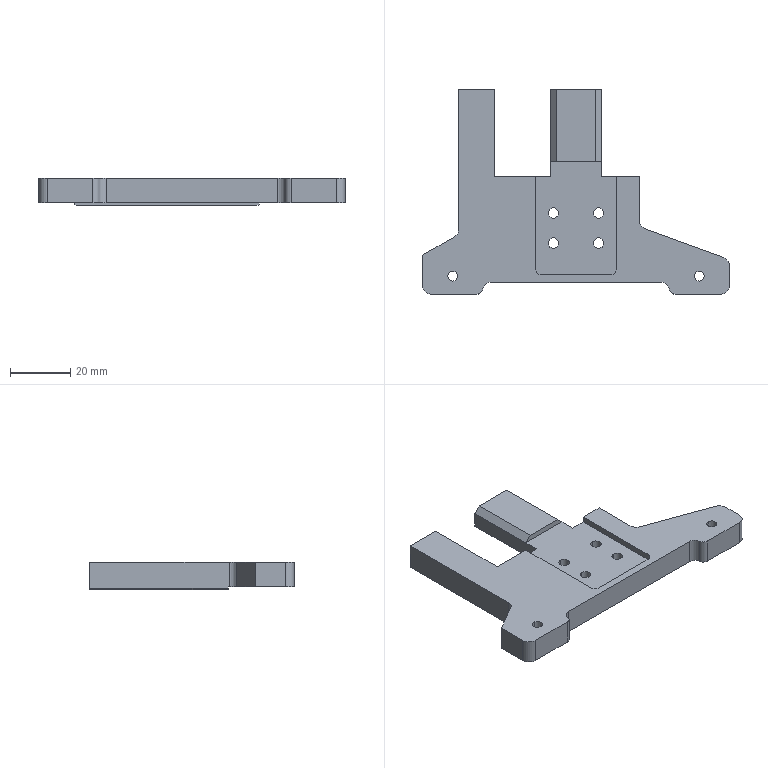NC program | NX | posted with a generic post | part box 102 x 68 x 9.2 mm
Whole program:
N10 G17 G21 G94 G90
(ZLEVEL_PROFILE_COPY_1 , TOOL : D4)
N12 T04 M6
N14 G54
N16 G17 G0 G90 X-43.633 Y-13.513 S7000 M3
N18 G43 Z11. H4
N20 Z-0.5
N22 G94 G1 X-43.033 Y-13.86 F1000.
N24 G3 X-42.633 Y-13.86 R0.4
N26 G1 X-41.5 Y-13.206 F1500.
N28 G3 X-41. Y-12.34 R1.
N30 G1 Y-11.032
N32 G3 X-41.2 Y-10.686 R0.4
N34 G1 X-41.8 Y-10.339
N36 G0 X-43.633 Y-13.513 Z-1.
N38 G1 X-43.033 Y-13.86 F1000.
N40 G3 X-42.633 Y-13.86 R0.4
N42 G1 X-41.5 Y-13.206 F1500.
N44 G3 X-41. Y-12.34 R1.
N46 G1 Y-11.032
N48 G3 X-41.2 Y-10.686 R0.4
N50 G1 X-41.8 Y-10.339
N52 G0 X-43.633 Y-13.513 Z-1.5
N54 G1 X-43.033 Y-13.86 F1000.
N56 G3 X-42.633 Y-13.86 R0.4
N58 G1 X-41.5 Y-13.206 F1500.
N60 G3 X-41. Y-12.34 R1.
N62 G1 Y-11.032
N64 G3 X-41.2 Y-10.686 R0.4
N66 G1 X-41.8 Y-10.339
N68 G0 X-43.633 Y-13.513 Z-2.
N70 G1 X-43.033 Y-13.86 F1000.
N72 G3 X-42.633 Y-13.86 R0.4
N74 G1 X-41.5 Y-13.206 F1500.
N76 G3 X-41. Y-12.34 R1.
N78 G1 Y-11.032
N80 G3 X-41.2 Y-10.686 R0.4
N82 G1 X-41.8 Y-10.339
N84 G0 X-43.633 Y-13.513 Z-2.48
N86 G1 X-43.033 Y-13.86 F1000.
N88 G3 X-42.633 Y-13.86 R0.4
N90 G1 X-41.5 Y-13.206 F1500.
N92 G3 X-41. Y-12.34 R1.
N94 G1 Y-11.032
N96 G3 X-41.2 Y-10.686 R0.4
N98 G1 X-41.8 Y-10.339
N100 G0 X-43.633 Y-13.513 Z-2.96
N102 G1 X-43.033 Y-13.86 F1000.
N104 G3 X-42.633 Y-13.86 R0.4
N106 G1 X-41.5 Y-13.206 F1500.
N108 G3 X-41. Y-12.34 R1.
N110 G1 Y-11.032
N112 G3 X-41.2 Y-10.686 R0.4
N114 G1 X-41.8 Y-10.339
N116 G0 X-43.633 Y-13.513 Z-3.44
N118 G1 X-43.033 Y-13.86 F1000.
N120 G3 X-42.633 Y-13.86 R0.4
N122 G1 X-41.5 Y-13.206 F1500.
N124 G3 X-41. Y-12.34 R1.
N126 G1 Y-11.032
N128 G3 X-41.2 Y-10.686 R0.4
N130 G1 X-41.8 Y-10.339
N132 G0 X-43.633 Y-13.513 Z-3.92
N134 G1 X-43.033 Y-13.86 F1000.
N136 G3 X-42.633 Y-13.86 R0.4
N138 G1 X-41.5 Y-13.206 F1500.
N140 G3 X-41. Y-12.34 R1.
N142 G1 Y-11.032
N144 G3 X-41.2 Y-10.686 R0.4
N146 G1 X-41.8 Y-10.339
N148 G0 X-43.633 Y-13.513 Z-4.4
N150 G1 X-43.033 Y-13.86 F1000.
N152 G3 X-42.633 Y-13.86 R0.4
N154 G1 X-41.5 Y-13.206 F1500.
N156 G3 X-41. Y-12.34 R1.
N158 G1 Y-11.032
N160 G3 X-41.2 Y-10.686 R0.4
N162 G1 X-41.8 Y-10.339
N164 G0 X-43.633 Y-13.513 Z-4.88
N166 G1 X-43.033 Y-13.86 F1000.
N168 G3 X-42.633 Y-13.86 R0.4
N170 G1 X-41.5 Y-13.206 F1500.
N172 G3 X-41. Y-12.34 R1.
N174 G1 Y-11.032
N176 G3 X-41.2 Y-10.686 R0.4
N178 G1 X-41.8 Y-10.339
N180 G0 X-43.633 Y-13.513 Z-5.36
N182 G1 X-43.033 Y-13.86 F1000.
N184 G3 X-42.633 Y-13.86 R0.4
N186 G1 X-41.5 Y-13.206 F1500.
N188 G3 X-41. Y-12.34 R1.
N190 G1 Y-11.032
N192 G3 X-41.2 Y-10.686 R0.4
N194 G1 X-41.8 Y-10.339
N196 G0 X-43.633 Y-13.513 Z-5.84
N198 G1 X-43.033 Y-13.86 F1000.
N200 G3 X-42.633 Y-13.86 R0.4
N202 G1 X-41.5 Y-13.206 F1500.
N204 G3 X-41. Y-12.34 R1.
N206 G1 Y-11.032
N208 G3 X-41.2 Y-10.686 R0.4
N210 G1 X-41.8 Y-10.339
N212 G0 X-43.633 Y-13.513 Z-6.32
N214 G1 X-43.033 Y-13.86 F1000.
N216 G3 X-42.633 Y-13.86 R0.4
N218 G1 X-41.5 Y-13.206 F1500.
N220 G3 X-41. Y-12.34 R1.
N222 G1 Y-11.032
N224 G3 X-41.2 Y-10.686 R0.4
N226 G1 X-41.8 Y-10.339
N228 G0 X-43.633 Y-13.513 Z-6.8
N230 G1 X-43.033 Y-13.86 F1000.
N232 G3 X-42.633 Y-13.86 R0.4
N234 G1 X-41.5 Y-13.206 F1500.
N236 G3 X-41. Y-12.34 R1.
N238 G1 Y-11.032
N240 G3 X-41.2 Y-10.686 R0.4
N242 G1 X-41.8 Y-10.339
N244 G0 X-43.633 Y-13.513 Z-7.28
N246 G1 X-43.033 Y-13.86 F1000.
N248 G3 X-42.633 Y-13.86 R0.4
N250 G1 X-41.5 Y-13.206 F1500.
N252 G3 X-41. Y-12.34 R1.
N254 G1 Y-11.032
N256 G3 X-41.2 Y-10.686 R0.4
N258 G1 X-41.8 Y-10.339
N260 G0 X-43.633 Y-13.513 Z-7.76
N262 G1 X-43.033 Y-13.86 F1000.
N264 G3 X-42.633 Y-13.86 R0.4
N266 G1 X-41.5 Y-13.206 F1500.
N268 G3 X-41. Y-12.34 R1.
N270 G1 Y-11.032
N272 G3 X-41.2 Y-10.686 R0.4
N274 G1 X-41.8 Y-10.339
N276 G0 X-43.633 Y-13.513 Z-8.24
N278 G1 X-43.033 Y-13.86 F1000.
N280 G3 X-42.633 Y-13.86 R0.4
N282 G1 X-41.5 Y-13.206 F1500.
N284 G3 X-41. Y-12.34 R1.
N286 G1 Y-11.032
N288 G3 X-41.2 Y-10.686 R0.4
N290 G1 X-41.8 Y-10.339
N292 G0 X-43.637 Y-13.516 Z-8.72
N294 G1 X-43.037 Y-13.862 F1000.
N296 G3 X-42.637 Y-13.862 R0.4
N298 G1 X-41.5 Y-13.206 F1500.
N300 G3 X-41. Y-12.34 R1.
N302 G1 Y-11.031
N304 G3 X-41.2 Y-10.685 R0.4
N306 G1 X-41.8 Y-10.339
N308 G0 X-43.637 Y-13.516 Z-9.2
N310 G1 X-43.037 Y-13.862 F1000.
N312 G3 X-42.637 Y-13.862 R0.4
N314 G1 X-41.5 Y-13.206 F1500.
N316 G3 X-41. Y-12.34 R1.
N318 G1 Y-11.031
N320 G3 X-41.2 Y-10.685 R0.4
N322 G1 X-41.8 Y-10.339
N324 G0 Z11.
N326 X-24.2 Y10.846
N328 Z-0.5
N330 G1 X-24.8 Y10.499 F1000.
N332 G3 X-25. Y10.153 R0.4
N334 G1 Y7. F1500.
N336 X-21.847
N338 G3 X-21.501 Y7.2 R0.4
N340 G1 X-21.154 Y7.8
N342 G0 X-24.2 Y10.846 Z-1.
N344 G1 X-24.8 Y10.499 F1000.
N346 G3 X-25. Y10.153 R0.4
N348 G1 Y7. F1500.
N350 X-21.847
N352 G3 X-21.501 Y7.2 R0.4
N354 G1 X-21.154 Y7.8
N356 G0 X-24.2 Y10.846 Z-1.5
N358 G1 X-24.8 Y10.499 F1000.
N360 G3 X-25. Y10.153 R0.4
N362 G1 Y7. F1500.
N364 X-21.847
N366 G3 X-21.501 Y7.2 R0.4
N368 G1 X-21.154 Y7.8
N370 G0 X-24.2 Y10.846 Z-2.
N372 G1 X-24.8 Y10.499 F1000.
N374 G3 X-25. Y10.153 R0.4
N376 G1 Y7. F1500.
N378 X-21.847
N380 G3 X-21.501 Y7.2 R0.4
N382 G1 X-21.154 Y7.8
N384 G0 X-24.2 Y10.846 Z-2.48
N386 G1 X-24.8 Y10.499 F1000.
N388 G3 X-25. Y10.153 R0.4
N390 G1 Y7. F1500.
N392 X-21.847
N394 G3 X-21.501 Y7.2 R0.4
N396 G1 X-21.154 Y7.8
N398 G0 X-24.2 Y10.846 Z-2.96
N400 G1 X-24.8 Y10.499 F1000.
N402 G3 X-25. Y10.153 R0.4
N404 G1 Y7. F1500.
N406 X-21.847
N408 G3 X-21.501 Y7.2 R0.4
N410 G1 X-21.154 Y7.8
N412 G0 X-24.2 Y10.846 Z-3.44
N414 G1 X-24.8 Y10.499 F1000.
N416 G3 X-25. Y10.153 R0.4
N418 G1 Y7. F1500.
N420 X-21.847
N422 G3 X-21.501 Y7.2 R0.4
N424 G1 X-21.154 Y7.8
N426 G0 X-24.2 Y10.846 Z-3.92
N428 G1 X-24.8 Y10.499 F1000.
N430 G3 X-25. Y10.153 R0.4
N432 G1 Y7. F1500.
N434 X-21.847
N436 G3 X-21.501 Y7.2 R0.4
N438 G1 X-21.154 Y7.8
N440 G0 X-24.2 Y10.846 Z-4.4
N442 G1 X-24.8 Y10.499 F1000.
N444 G3 X-25. Y10.153 R0.4
N446 G1 Y7. F1500.
N448 X-21.847
N450 G3 X-21.501 Y7.2 R0.4
N452 G1 X-21.154 Y7.8
N454 G0 X-24.2 Y10.846 Z-4.88
N456 G1 X-24.8 Y10.499 F1000.
N458 G3 X-25. Y10.153 R0.4
N460 G1 Y7. F1500.
N462 X-21.847
N464 G3 X-21.501 Y7.2 R0.4
N466 G1 X-21.154 Y7.8
N468 G0 X-24.2 Y10.846 Z-5.36
N470 G1 X-24.8 Y10.499 F1000.
N472 G3 X-25. Y10.153 R0.4
N474 G1 Y7. F1500.
N476 X-21.847
N478 G3 X-21.501 Y7.2 R0.4
N480 G1 X-21.154 Y7.8
N482 G0 X-24.2 Y10.846 Z-5.84
N484 G1 X-24.8 Y10.499 F1000.
N486 G3 X-25. Y10.153 R0.4
N488 G1 Y7. F1500.
N490 X-21.847
N492 G3 X-21.501 Y7.2 R0.4
N494 G1 X-21.154 Y7.8
N496 G0 X-24.2 Y10.846 Z-6.32
N498 G1 X-24.8 Y10.499 F1000.
N500 G3 X-25. Y10.153 R0.4
N502 G1 Y7. F1500.
N504 X-21.847
N506 G3 X-21.501 Y7.2 R0.4
N508 G1 X-21.154 Y7.8
N510 G0 X-24.2 Y10.846 Z-6.8
N512 G1 X-24.8 Y10.499 F1000.
N514 G3 X-25. Y10.153 R0.4
N516 G1 Y7. F1500.
N518 X-21.847
N520 G3 X-21.501 Y7.2 R0.4
N522 G1 X-21.154 Y7.8
N524 G0 X-24.2 Y10.846 Z-7.28
N526 G1 X-24.8 Y10.499 F1000.
N528 G3 X-25. Y10.153 R0.4
N530 G1 Y7. F1500.
N532 X-21.847
N534 G3 X-21.501 Y7.2 R0.4
N536 G1 X-21.154 Y7.8
N538 G0 X-24.2 Y10.846 Z-7.76
N540 G1 X-24.8 Y10.499 F1000.
N542 G3 X-25. Y10.153 R0.4
N544 G1 Y7. F1500.
N546 X-21.847
N548 G3 X-21.501 Y7.2 R0.4
N550 G1 X-21.154 Y7.8
N552 G0 X-24.2 Y10.846 Z-8.24
N554 G1 X-24.8 Y10.499 F1000.
N556 G3 X-25. Y10.153 R0.4
N558 G1 Y7. F1500.
N560 X-21.847
N562 G3 X-21.501 Y7.2 R0.4
N564 G1 X-21.154 Y7.8
N566 G0 X-24.2 Y10.846 Z-8.72
N568 G1 X-24.8 Y10.499 F1000.
N570 G3 X-25. Y10.153 R0.4
N572 G1 Y7. F1500.
N574 X-21.847
N576 G3 X-21.501 Y7.2 R0.4
N578 G1 X-21.154 Y7.8
N580 G0 X-24.2 Y10.846 Z-9.2
N582 G1 X-24.8 Y10.499 F1000.
N584 G3 X-25. Y10.153 R0.4
N586 G1 Y7. F1500.
N588 X-21.847
N590 G3 X-21.501 Y7.2 R0.4
N592 G1 X-21.154 Y7.8
N594 G0 Z11.
N596 X-10.7 Y-21.654
N598 Z-0.5
N600 G1 X-11.3 Y-22.001 F1000.
N602 G3 X-11.5 Y-22.347 R0.4
N604 G1 Y-25.5 F1500.
N606 X-8.347
N608 G3 X-8.001 Y-25.3 R0.4
N610 G1 X-7.654 Y-24.7
N612 G0 X-10.7 Y-21.654 Z-1.
N614 G1 X-11.3 Y-22.001 F1000.
N616 G3 X-11.5 Y-22.347 R0.4
N618 G1 Y-25.5 F1500.
N620 X-8.347
N622 G3 X-8.001 Y-25.3 R0.4
N624 G1 X-7.654 Y-24.7
N626 G0 X-10.7 Y-21.654 Z-1.5
N628 G1 X-11.3 Y-22.001 F1000.
N630 G3 X-11.5 Y-22.347 R0.4
N632 G1 Y-25.5 F1500.
N634 X-8.347
N636 G3 X-8.001 Y-25.3 R0.4
N638 G1 X-7.654 Y-24.7
N640 G0 X-10.7 Y-21.654 Z-2.
N642 G1 X-11.3 Y-22.001 F1000.
N644 G3 X-11.5 Y-22.347 R0.4
N646 G1 X-11.499 Y-25.5 F1500.
N648 X-8.347
N650 G3 X-8.001 Y-25.3 R0.4
N652 G1 X-7.654 Y-24.7
N654 G0 Z11.
N656 X7.654
N658 Z-0.5
N660 G1 X8. Y-25.3 F1000.
N662 G3 X8.347 Y-25.5 R0.4
N664 G1 X11.5 F1500.
N666 Y-22.347
N668 G3 X11.3 Y-22. R0.4
N670 G1 X10.7 Y-21.654
N672 G0 X7.654 Y-24.7 Z-1.
N674 G1 X8. Y-25.3 F1000.
N676 G3 X8.346 Y-25.5 R0.4
N678 G1 X11.5 F1500.
N680 Y-22.346
N682 G3 X11.3 Y-22. R0.4
N684 G1 X10.7 Y-21.654
N686 G0 X7.653 Y-24.7 Z-1.5
N688 G1 X8. Y-25.3 F1000.
N690 G3 X8.346 Y-25.5 R0.4
N692 G1 X11.5 F1500.
N694 Y-22.346
N696 G3 X11.3 Y-22. R0.4
N698 G1 X10.7 Y-21.653
N700 G0 X7.653 Y-24.7 Z-2.
N702 G1 X7.999 Y-25.3 F1000.
N704 G3 X8.346 Y-25.5 R0.4
N706 G1 X11.5 F1500.
N708 Y-22.346
N710 G3 X11.3 Y-21.999 R0.4
N712 G1 X10.7 Y-21.653
N714 G0 Z11.
N716 X23.8 Y-7.234
N718 Z-0.5
N720 G1 X23.2 Y-7.58 F1000.
N722 G3 X23. Y-7.927 R0.4
N724 G1 Y-9.48 F1500.
N726 G3 X23.658 Y-10.42 R1.
N728 G1 X25.118 Y-10.951
N730 G3 X25.512 Y-10.882 R0.4
N732 G1 X26.042 Y-10.436
N734 G0 X23.8 Y-7.234 Z-1.
N736 G1 X23.2 Y-7.58 F1000.
N738 G3 X23. Y-7.927 R0.4
N740 G1 Y-9.48 F1500.
N742 G3 X23.658 Y-10.42 R1.
N744 G1 X25.118 Y-10.951
N746 G3 X25.512 Y-10.882 R0.4
N748 G1 X26.042 Y-10.436
N750 G0 X23.8 Y-7.234 Z-1.5
N752 G1 X23.2 Y-7.58 F1000.
N754 G3 X23. Y-7.927 R0.4
N756 G1 Y-9.48 F1500.
N758 G3 X23.658 Y-10.42 R1.
N760 G1 X25.118 Y-10.951
N762 G3 X25.512 Y-10.882 R0.4
N764 G1 X26.042 Y-10.436
N766 G0 X23.8 Y-7.234 Z-2.
N768 G1 X23.2 Y-7.58 F1000.
N770 G3 X23. Y-7.927 R0.4
N772 G1 Y-9.48 F1500.
N774 G3 X23.658 Y-10.42 R1.
N776 G1 X25.118 Y-10.951
N778 G3 X25.512 Y-10.882 R0.4
N780 G1 X26.042 Y-10.436
N782 G0 X23.8 Y-7.234 Z-2.48
N784 G1 X23.2 Y-7.58 F1000.
N786 G3 X23. Y-7.927 R0.4
N788 G1 Y-9.48 F1500.
N790 G3 X23.658 Y-10.42 R1.
N792 G1 X25.118 Y-10.951
N794 G3 X25.512 Y-10.882 R0.4
N796 G1 X26.042 Y-10.436
N798 G0 X23.8 Y-7.234 Z-2.96
N800 G1 X23.2 Y-7.58 F1000.
N802 G3 X23. Y-7.927 R0.4
N804 G1 Y-9.48 F1500.
N806 G3 X23.658 Y-10.42 R1.
N808 G1 X25.118 Y-10.951
N810 G3 X25.512 Y-10.882 R0.4
N812 G1 X26.042 Y-10.436
N814 G0 X23.8 Y-7.234 Z-3.44
N816 G1 X23.2 Y-7.58 F1000.
N818 G3 X23. Y-7.927 R0.4
N820 G1 Y-9.48 F1500.
N822 G3 X23.658 Y-10.42 R1.
N824 G1 X25.118 Y-10.951
N826 G3 X25.512 Y-10.882 R0.4
N828 G1 X26.042 Y-10.436
N830 G0 X23.8 Y-7.234 Z-3.92
N832 G1 X23.2 Y-7.58 F1000.
N834 G3 X23. Y-7.927 R0.4
N836 G1 Y-9.48 F1500.
N838 G3 X23.658 Y-10.42 R1.
N840 G1 X25.118 Y-10.951
N842 G3 X25.512 Y-10.882 R0.4
N844 G1 X26.042 Y-10.436
N846 G0 X23.8 Y-7.234 Z-4.4
N848 G1 X23.2 Y-7.58 F1000.
N850 G3 X23. Y-7.927 R0.4
N852 G1 Y-9.48 F1500.
N854 G3 X23.658 Y-10.42 R1.
N856 G1 X25.118 Y-10.951
N858 G3 X25.512 Y-10.882 R0.4
N860 G1 X26.042 Y-10.436
N862 G0 X23.8 Y-7.234 Z-4.88
N864 G1 X23.2 Y-7.58 F1000.
N866 G3 X23. Y-7.927 R0.4
N868 G1 Y-9.48 F1500.
N870 G3 X23.658 Y-10.42 R1.
N872 G1 X25.118 Y-10.951
N874 G3 X25.512 Y-10.882 R0.4
N876 G1 X26.042 Y-10.436
N878 G0 X23.8 Y-7.234 Z-5.36
N880 G1 X23.2 Y-7.58 F1000.
N882 G3 X23. Y-7.927 R0.4
N884 G1 Y-9.48 F1500.
N886 G3 X23.658 Y-10.42 R1.
N888 G1 X25.118 Y-10.951
N890 G3 X25.512 Y-10.882 R0.4
N892 G1 X26.042 Y-10.436
N894 G0 X23.8 Y-7.234 Z-5.84
N896 G1 X23.2 Y-7.58 F1000.
N898 G3 X23. Y-7.927 R0.4
N900 G1 Y-9.48 F1500.
N902 G3 X23.658 Y-10.42 R1.
N904 G1 X25.118 Y-10.951
N906 G3 X25.512 Y-10.882 R0.4
N908 G1 X26.042 Y-10.436
N910 G0 X23.8 Y-7.234 Z-6.32
N912 G1 X23.2 Y-7.58 F1000.
N914 G3 X23. Y-7.927 R0.4
N916 G1 Y-9.48 F1500.
N918 G3 X23.658 Y-10.42 R1.
N920 G1 X25.118 Y-10.951
N922 G3 X25.512 Y-10.882 R0.4
N924 G1 X26.042 Y-10.436
N926 G0 X23.8 Y-7.234 Z-6.8
N928 G1 X23.2 Y-7.58 F1000.
N930 G3 X23. Y-7.927 R0.4
N932 G1 Y-9.48 F1500.
N934 G3 X23.658 Y-10.42 R1.
N936 G1 X25.118 Y-10.951
N938 G3 X25.512 Y-10.882 R0.4
N940 G1 X26.042 Y-10.436
N942 G0 X23.8 Y-7.234 Z-7.28
N944 G1 X23.2 Y-7.58 F1000.
N946 G3 X23. Y-7.927 R0.4
N948 G1 Y-9.48 F1500.
N950 G3 X23.658 Y-10.42 R1.
N952 G1 X25.118 Y-10.951
N954 G3 X25.512 Y-10.882 R0.4
N956 G1 X26.042 Y-10.436
N958 G0 X23.8 Y-7.234 Z-7.76
N960 G1 X23.2 Y-7.58 F1000.
N962 G3 X23. Y-7.927 R0.4
N964 G1 Y-9.48 F1500.
N966 G3 X23.658 Y-10.42 R1.
N968 G1 X25.118 Y-10.951
N970 G3 X25.512 Y-10.882 R0.4
N972 G1 X26.042 Y-10.436
N974 G0 X23.8 Y-7.234 Z-8.24
N976 G1 X23.2 Y-7.58 F1000.
N978 G3 X23. Y-7.927 R0.4
N980 G1 Y-9.48 F1500.
N982 G3 X23.658 Y-10.42 R1.
N984 G1 X25.118 Y-10.951
N986 G3 X25.512 Y-10.882 R0.4
N988 G1 X26.042 Y-10.436
N990 G0 X23.8 Y-7.234 Z-8.72
N992 G1 X23.2 Y-7.58 F1000.
N994 G3 X23. Y-7.927 R0.4
N996 G1 Y-9.48 F1500.
N998 G3 X23.658 Y-10.42 R1.
N1000 G1 X25.118 Y-10.951
N1002 G3 X25.512 Y-10.882 R0.4
N1004 G1 X26.042 Y-10.436
N1006 G0 X23.8 Y-7.234 Z-9.2
N1008 G1 X23.2 Y-7.58 F1000.
N1010 G3 X23. Y-7.927 R0.4
N1012 G1 Y-9.48 F1500.
N1014 G3 X23.658 Y-10.42 R1.
N1016 G1 X25.118 Y-10.951
N1018 G3 X25.512 Y-10.882 R0.4
N1020 G1 X26.042 Y-10.436
N1022 G0 Z11.
N1024 X29.127 Y-34.873
N1026 Z-0.5
N1028 G1 X29.458 Y-34.326 F1000.
N1030 G3 X29.466 Y-33.926 R0.4
N1032 G2 X28.997 Y-32.444 R4. F1500.
N1034 G3 X28.5 Y-32. R0.5
N1036 G1 X26.495
N1038 G3 X26.148 Y-32.2 R0.4
N1040 G1 X25.802 Y-32.8
N1042 G0 X29.127 Y-34.873 Z-1.
N1044 G1 X29.458 Y-34.326 F1000.
N1046 G3 X29.466 Y-33.926 R0.4
N1048 G2 X28.997 Y-32.444 R4. F1500.
N1050 G3 X28.5 Y-32. R0.5
N1052 G1 X26.495
N1054 G3 X26.148 Y-32.2 R0.4
N1056 G1 X25.802 Y-32.8
N1058 G0 X29.127 Y-34.873 Z-1.5
N1060 G1 X29.458 Y-34.326 F1000.
N1062 G3 X29.466 Y-33.926 R0.4
N1064 G2 X28.997 Y-32.444 R4. F1500.
N1066 G3 X28.5 Y-32. R0.5
N1068 G1 X26.495
N1070 G3 X26.148 Y-32.2 R0.4
N1072 G1 X25.802 Y-32.8
N1074 G0 X29.127 Y-34.873 Z-2.
N1076 G1 X29.458 Y-34.326 F1000.
N1078 G3 X29.466 Y-33.926 R0.4
N1080 G2 X28.997 Y-32.444 R4. F1500.
N1082 G3 X28.5 Y-32. R0.5
N1084 G1 X26.495
N1086 G3 X26.148 Y-32.2 R0.4
N1088 G1 X25.802 Y-32.8
N1090 G0 X29.127 Y-34.873 Z-2.48
N1092 G1 X29.458 Y-34.326 F1000.
N1094 G3 X29.466 Y-33.926 R0.4
N1096 G2 X28.997 Y-32.444 R4. F1500.
N1098 G3 X28.5 Y-32. R0.5
N1100 G1 X26.495
N1102 G3 X26.148 Y-32.2 R0.4
N1104 G1 X25.802 Y-32.8
N1106 G0 X29.127 Y-34.873 Z-2.96
N1108 G1 X29.458 Y-34.326 F1000.
N1110 G3 X29.466 Y-33.926 R0.4
N1112 G2 X28.997 Y-32.444 R4. F1500.
N1114 G3 X28.5 Y-32. R0.5
N1116 G1 X26.495
N1118 G3 X26.148 Y-32.2 R0.4
N1120 G1 X25.802 Y-32.8
N1122 G0 X29.127 Y-34.873 Z-3.44
N1124 G1 X29.458 Y-34.326 F1000.
N1126 G3 X29.466 Y-33.926 R0.4
N1128 G2 X28.997 Y-32.444 R4. F1500.
N1130 G3 X28.5 Y-32. R0.5
N1132 G1 X26.495
N1134 G3 X26.148 Y-32.2 R0.4
N1136 G1 X25.802 Y-32.8
N1138 G0 X29.127 Y-34.873 Z-3.92
N1140 G1 X29.458 Y-34.326 F1000.
N1142 G3 X29.466 Y-33.926 R0.4
N1144 G2 X28.997 Y-32.444 R4. F1500.
N1146 G3 X28.5 Y-32. R0.5
N1148 G1 X26.495
N1150 G3 X26.148 Y-32.2 R0.4
N1152 G1 X25.802 Y-32.8
N1154 G0 X29.127 Y-34.873 Z-4.4
N1156 G1 X29.458 Y-34.326 F1000.
N1158 G3 X29.466 Y-33.926 R0.4
N1160 G2 X28.997 Y-32.444 R4. F1500.
N1162 G3 X28.5 Y-32. R0.5
N1164 G1 X26.495
N1166 G3 X26.148 Y-32.2 R0.4
N1168 G1 X25.802 Y-32.8
N1170 G0 X29.127 Y-34.873 Z-4.88
N1172 G1 X29.458 Y-34.326 F1000.
N1174 G3 X29.466 Y-33.926 R0.4
N1176 G2 X28.997 Y-32.444 R4. F1500.
N1178 G3 X28.5 Y-32. R0.5
N1180 G1 X26.495
N1182 G3 X26.148 Y-32.2 R0.4
N1184 G1 X25.802 Y-32.8
N1186 G0 X29.127 Y-34.873 Z-5.36
N1188 G1 X29.458 Y-34.326 F1000.
N1190 G3 X29.466 Y-33.926 R0.4
N1192 G2 X28.997 Y-32.444 R4. F1500.
N1194 G3 X28.5 Y-32. R0.5
N1196 G1 X26.495
N1198 G3 X26.148 Y-32.2 R0.4
N1200 G1 X25.802 Y-32.8
N1202 G0 X29.127 Y-34.873 Z-5.84
N1204 G1 X29.458 Y-34.326 F1000.
N1206 G3 X29.466 Y-33.926 R0.4
N1208 G2 X28.997 Y-32.444 R4. F1500.
N1210 G3 X28.5 Y-32. R0.5
N1212 G1 X26.495
N1214 G3 X26.148 Y-32.2 R0.4
N1216 G1 X25.802 Y-32.8
N1218 G0 X29.127 Y-34.873 Z-6.32
N1220 G1 X29.458 Y-34.326 F1000.
N1222 G3 X29.466 Y-33.926 R0.4
N1224 G2 X28.997 Y-32.444 R4. F1500.
N1226 G3 X28.5 Y-32. R0.5
N1228 G1 X26.495
N1230 G3 X26.148 Y-32.2 R0.4
N1232 G1 X25.802 Y-32.8
N1234 G0 X29.127 Y-34.873 Z-6.8
N1236 G1 X29.458 Y-34.326 F1000.
N1238 G3 X29.466 Y-33.926 R0.4
N1240 G2 X28.997 Y-32.444 R4. F1500.
N1242 G3 X28.5 Y-32. R0.5
N1244 G1 X26.495
N1246 G3 X26.148 Y-32.2 R0.4
N1248 G1 X25.802 Y-32.8
N1250 G0 X29.127 Y-34.873 Z-7.28
N1252 G1 X29.458 Y-34.326 F1000.
N1254 G3 X29.466 Y-33.926 R0.4
N1256 G2 X28.997 Y-32.444 R4. F1500.
N1258 G3 X28.5 Y-32. R0.5
N1260 G1 X26.495
N1262 G3 X26.148 Y-32.2 R0.4
N1264 G1 X25.802 Y-32.8
N1266 G0 X29.127 Y-34.873 Z-7.76
N1268 G1 X29.458 Y-34.326 F1000.
N1270 G3 X29.466 Y-33.926 R0.4
N1272 G2 X28.997 Y-32.444 R4. F1500.
N1274 G3 X28.5 Y-32. R0.5
N1276 G1 X26.495
N1278 G3 X26.148 Y-32.2 R0.4
N1280 G1 X25.802 Y-32.8
N1282 G0 X29.12 Y-34.864 Z-8.24
N1284 G1 X29.452 Y-34.318 F1000.
N1286 G3 X29.462 Y-33.918 R0.4
N1288 G2 X28.997 Y-32.444 R4. F1500.
N1290 G3 X28.5 Y-32. R0.5
N1292 G1 X26.508
N1294 G3 X26.161 Y-32.2 R0.4
N1296 G1 X25.815 Y-32.8
N1298 G0 X29.12 Y-34.864 Z-8.72
N1300 G1 X29.452 Y-34.318 F1000.
N1302 G3 X29.462 Y-33.918 R0.4
N1304 G2 X28.997 Y-32.444 R4. F1500.
N1306 G3 X28.5 Y-32. R0.5
N1308 G1 X26.508
N1310 G3 X26.161 Y-32.2 R0.4
N1312 G1 X25.815 Y-32.8
N1314 G0 X29.12 Y-34.864 Z-9.2
N1316 G1 X29.452 Y-34.318 F1000.
N1318 G3 X29.462 Y-33.918 R0.4
N1320 G2 X28.997 Y-32.444 R4. F1500.
N1322 G3 X28.5 Y-32. R0.5
N1324 G1 X26.508
N1326 G3 X26.161 Y-32.2 R0.4
N1328 G1 X25.815 Y-32.8
N1330 G0 Z11.
N1332 X-25.802
N1334 Z-0.5
N1336 G1 X-26.148 Y-32.2 F1000.
N1338 G3 X-26.495 Y-32. R0.4
N1340 G1 X-28.5 F1500.
N1342 G3 X-28.997 Y-32.444 R0.5
N1344 G2 X-29.466 Y-33.926 R4.
N1346 G3 X-29.458 Y-34.326 R0.4
N1348 G1 X-29.127 Y-34.873
N1350 G0 X-25.802 Y-32.8 Z-1.
N1352 G1 X-26.148 Y-32.2 F1000.
N1354 G3 X-26.495 Y-32. R0.4
N1356 G1 X-28.5 F1500.
N1358 G3 X-28.997 Y-32.444 R0.5
N1360 G2 X-29.466 Y-33.926 R4.
N1362 G3 X-29.458 Y-34.326 R0.4
N1364 G1 X-29.127 Y-34.873
N1366 G0 X-25.802 Y-32.8 Z-1.5
N1368 G1 X-26.148 Y-32.2 F1000.
N1370 G3 X-26.495 Y-32. R0.4
N1372 G1 X-28.5 F1500.
N1374 G3 X-28.997 Y-32.444 R0.5
N1376 G2 X-29.466 Y-33.926 R4.
N1378 G3 X-29.458 Y-34.326 R0.4
N1380 G1 X-29.127 Y-34.873
N1382 G0 X-25.802 Y-32.8 Z-2.
N1384 G1 X-26.148 Y-32.2 F1000.
N1386 G3 X-26.495 Y-32. R0.4
N1388 G1 X-28.5 F1500.
N1390 G3 X-28.997 Y-32.444 R0.5
N1392 G2 X-29.466 Y-33.926 R4.
N1394 G3 X-29.458 Y-34.326 R0.4
N1396 G1 X-29.127 Y-34.873
N1398 G0 X-25.802 Y-32.8 Z-2.48
N1400 G1 X-26.148 Y-32.2 F1000.
N1402 G3 X-26.495 Y-32. R0.4
N1404 G1 X-28.5 F1500.
N1406 G3 X-28.997 Y-32.444 R0.5
N1408 G2 X-29.466 Y-33.926 R4.
N1410 G3 X-29.458 Y-34.326 R0.4
N1412 G1 X-29.127 Y-34.873
N1414 G0 X-25.802 Y-32.8 Z-2.96
N1416 G1 X-26.148 Y-32.2 F1000.
N1418 G3 X-26.495 Y-32. R0.4
N1420 G1 X-28.5 F1500.
N1422 G3 X-28.997 Y-32.444 R0.5
N1424 G2 X-29.466 Y-33.926 R4.
N1426 G3 X-29.458 Y-34.326 R0.4
N1428 G1 X-29.127 Y-34.873
N1430 G0 X-25.802 Y-32.8 Z-3.44
N1432 G1 X-26.148 Y-32.2 F1000.
N1434 G3 X-26.495 Y-32. R0.4
N1436 G1 X-28.5 F1500.
N1438 G3 X-28.997 Y-32.444 R0.5
N1440 G2 X-29.466 Y-33.926 R4.
N1442 G3 X-29.458 Y-34.326 R0.4
N1444 G1 X-29.127 Y-34.873
N1446 G0 X-25.802 Y-32.8 Z-3.92
N1448 G1 X-26.148 Y-32.2 F1000.
N1450 G3 X-26.495 Y-32. R0.4
N1452 G1 X-28.5 F1500.
N1454 G3 X-28.997 Y-32.444 R0.5
N1456 G2 X-29.466 Y-33.926 R4.
N1458 G3 X-29.458 Y-34.326 R0.4
N1460 G1 X-29.127 Y-34.873
N1462 G0 X-25.802 Y-32.8 Z-4.4
N1464 G1 X-26.148 Y-32.2 F1000.
N1466 G3 X-26.495 Y-32. R0.4
N1468 G1 X-28.5 F1500.
N1470 G3 X-28.997 Y-32.444 R0.5
N1472 G2 X-29.466 Y-33.926 R4.
N1474 G3 X-29.458 Y-34.326 R0.4
N1476 G1 X-29.127 Y-34.873
N1478 G0 X-25.802 Y-32.8 Z-4.88
N1480 G1 X-26.148 Y-32.2 F1000.
N1482 G3 X-26.495 Y-32. R0.4
N1484 G1 X-28.5 F1500.
N1486 G3 X-28.997 Y-32.444 R0.5
N1488 G2 X-29.466 Y-33.926 R4.
N1490 G3 X-29.458 Y-34.326 R0.4
N1492 G1 X-29.127 Y-34.873
N1494 G0 X-25.802 Y-32.8 Z-5.36
N1496 G1 X-26.148 Y-32.2 F1000.
N1498 G3 X-26.495 Y-32. R0.4
N1500 G1 X-28.5 F1500.
N1502 G3 X-28.997 Y-32.444 R0.5
N1504 G2 X-29.466 Y-33.926 R4.
N1506 G3 X-29.458 Y-34.326 R0.4
N1508 G1 X-29.127 Y-34.873
N1510 G0 X-25.802 Y-32.8 Z-5.84
N1512 G1 X-26.148 Y-32.2 F1000.
N1514 G3 X-26.495 Y-32. R0.4
N1516 G1 X-28.5 F1500.
N1518 G3 X-28.997 Y-32.444 R0.5
N1520 G2 X-29.466 Y-33.926 R4.
N1522 G3 X-29.458 Y-34.326 R0.4
N1524 G1 X-29.127 Y-34.873
N1526 G0 X-25.802 Y-32.8 Z-6.32
N1528 G1 X-26.148 Y-32.2 F1000.
N1530 G3 X-26.495 Y-32. R0.4
N1532 G1 X-28.5 F1500.
N1534 G3 X-28.997 Y-32.444 R0.5
N1536 G2 X-29.466 Y-33.926 R4.
N1538 G3 X-29.458 Y-34.326 R0.4
N1540 G1 X-29.127 Y-34.873
N1542 G0 X-25.802 Y-32.8 Z-6.8
N1544 G1 X-26.148 Y-32.2 F1000.
N1546 G3 X-26.495 Y-32. R0.4
N1548 G1 X-28.5 F1500.
N1550 G3 X-28.997 Y-32.444 R0.5
N1552 G2 X-29.466 Y-33.926 R4.
N1554 G3 X-29.458 Y-34.326 R0.4
N1556 G1 X-29.127 Y-34.873
N1558 G0 X-25.802 Y-32.8 Z-7.28
N1560 G1 X-26.148 Y-32.2 F1000.
N1562 G3 X-26.495 Y-32. R0.4
N1564 G1 X-28.5 F1500.
N1566 G3 X-28.997 Y-32.444 R0.5
N1568 G2 X-29.466 Y-33.926 R4.
N1570 G3 X-29.458 Y-34.326 R0.4
N1572 G1 X-29.127 Y-34.873
N1574 G0 X-25.802 Y-32.8 Z-7.76
N1576 G1 X-26.148 Y-32.2 F1000.
N1578 G3 X-26.495 Y-32. R0.4
N1580 G1 X-28.5 F1500.
N1582 G3 X-28.997 Y-32.444 R0.5
N1584 G2 X-29.466 Y-33.926 R4.
N1586 G3 X-29.458 Y-34.326 R0.4
N1588 G1 X-29.127 Y-34.873
N1590 G0 X-25.815 Y-32.8 Z-8.24
N1592 G1 X-26.161 Y-32.2 F1000.
N1594 G3 X-26.508 Y-32. R0.4
N1596 G1 X-28.5 F1500.
N1598 G3 X-28.997 Y-32.444 R0.5
N1600 G2 X-29.462 Y-33.918 R4.
N1602 G3 X-29.452 Y-34.318 R0.4
N1604 G1 X-29.12 Y-34.864
N1606 G0 X-25.815 Y-32.8 Z-8.72
N1608 G1 X-26.161 Y-32.2 F1000.
N1610 G3 X-26.508 Y-32. R0.4
N1612 G1 X-28.5 F1500.
N1614 G3 X-28.997 Y-32.444 R0.5
N1616 G2 X-29.462 Y-33.918 R4.
N1618 G3 X-29.452 Y-34.318 R0.4
N1620 G1 X-29.12 Y-34.864
N1622 G0 X-25.815 Y-32.8 Z-9.2
N1624 G1 X-26.161 Y-32.2 F1000.
N1626 G3 X-26.508 Y-32. R0.4
N1628 G1 X-28.5 F1500.
N1630 G3 X-28.997 Y-32.444 R0.5
N1632 G2 X-29.462 Y-33.918 R4.
N1634 G3 X-29.452 Y-34.318 R0.4
N1636 G1 X-29.12 Y-34.864
N1638 G0 Z11.
N1640 X-14.345 Y7.8
N1642 Z-2.48
N1644 G1 X-13.998 Y7.2 F1000.
N1646 G3 X-13.652 Y7. R0.4
N1648 G1 X-10.5 F1500.
N1650 Y10.143
N1652 G3 X-10.7 Y10.489 R0.4
N1654 G1 X-11.3 Y10.836
N1656 G0 X-14.345 Y7.8 Z-2.96
N1658 G1 X-13.998 Y7.2 F1000.
N1660 G3 X-13.652 Y7. R0.4
N1662 G1 X-10.5 F1500.
N1664 Y10.143
N1666 G3 X-10.7 Y10.489 R0.4
N1668 G1 X-11.3 Y10.836
N1670 G0 X-14.345 Y7.8 Z-3.44
N1672 G1 X-13.998 Y7.2 F1000.
N1674 G3 X-13.652 Y7. R0.4
N1676 G1 X-10.5 F1500.
N1678 Y10.143
N1680 G3 X-10.7 Y10.489 R0.4
N1682 G1 X-11.3 Y10.836
N1684 G0 X-14.345 Y7.8 Z-3.92
N1686 G1 X-13.998 Y7.2 F1000.
N1688 G3 X-13.652 Y7. R0.4
N1690 G1 X-10.5 F1500.
N1692 Y10.143
N1694 G3 X-10.7 Y10.489 R0.4
N1696 G1 X-11.3 Y10.836
N1698 G0 X-14.345 Y7.8 Z-4.4
N1700 G1 X-13.998 Y7.2 F1000.
N1702 G3 X-13.652 Y7. R0.4
N1704 G1 X-10.5 F1500.
N1706 Y10.143
N1708 G3 X-10.7 Y10.489 R0.4
N1710 G1 X-11.3 Y10.836
N1712 G0 X-14.345 Y7.8 Z-4.88
N1714 G1 X-13.998 Y7.2 F1000.
N1716 G3 X-13.652 Y7. R0.4
N1718 G1 X-10.5 F1500.
N1720 Y10.143
N1722 G3 X-10.7 Y10.489 R0.4
N1724 G1 X-11.3 Y10.836
N1726 G0 X-14.345 Y7.8 Z-5.36
N1728 G1 X-13.998 Y7.2 F1000.
N1730 G3 X-13.652 Y7. R0.4
N1732 G1 X-10.5 F1500.
N1734 Y10.143
N1736 G3 X-10.7 Y10.489 R0.4
N1738 G1 X-11.3 Y10.836
N1740 G0 X-14.345 Y7.8 Z-5.84
N1742 G1 X-13.998 Y7.2 F1000.
N1744 G3 X-13.652 Y7. R0.4
N1746 G1 X-10.5 F1500.
N1748 Y10.143
N1750 G3 X-10.7 Y10.489 R0.4
N1752 G1 X-11.3 Y10.836
N1754 G0 X-14.345 Y7.8 Z-6.32
N1756 G1 X-13.998 Y7.2 F1000.
N1758 G3 X-13.652 Y7. R0.4
N1760 G1 X-10.5 F1500.
N1762 Y10.143
N1764 G3 X-10.7 Y10.489 R0.4
N1766 G1 X-11.3 Y10.836
N1768 G0 X-14.345 Y7.8 Z-6.8
N1770 G1 X-13.998 Y7.2 F1000.
N1772 G3 X-13.652 Y7. R0.4
N1774 G1 X-10.5 F1500.
N1776 Y10.143
N1778 G3 X-10.7 Y10.489 R0.4
N1780 G1 X-11.3 Y10.836
N1782 G0 X-14.345 Y7.8 Z-7.28
N1784 G1 X-13.998 Y7.2 F1000.
N1786 G3 X-13.652 Y7. R0.4
N1788 G1 X-10.5 F1500.
N1790 Y10.143
N1792 G3 X-10.7 Y10.489 R0.4
N1794 G1 X-11.3 Y10.836
N1796 G0 X-14.345 Y7.8 Z-7.76
N1798 G1 X-13.998 Y7.2 F1000.
N1800 G3 X-13.652 Y7. R0.4
N1802 G1 X-10.5 F1500.
N1804 Y10.143
N1806 G3 X-10.7 Y10.489 R0.4
N1808 G1 X-11.3 Y10.836
N1810 G0 X-14.345 Y7.8 Z-8.24
N1812 G1 X-13.998 Y7.2 F1000.
N1814 G3 X-13.652 Y7. R0.4
N1816 G1 X-10.5 F1500.
N1818 Y10.143
N1820 G3 X-10.7 Y10.489 R0.4
N1822 G1 X-11.3 Y10.836
N1824 G0 X-14.345 Y7.8 Z-8.72
N1826 G1 X-13.998 Y7.2 F1000.
N1828 G3 X-13.652 Y7. R0.4
N1830 G1 X-10.5 F1500.
N1832 Y10.143
N1834 G3 X-10.7 Y10.489 R0.4
N1836 G1 X-11.3 Y10.836
N1838 G0 X-14.345 Y7.8 Z-9.2
N1840 G1 X-13.998 Y7.2 F1000.
N1842 G3 X-13.652 Y7. R0.4
N1844 G1 X-10.5 F1500.
N1846 Y10.143
N1848 G3 X-10.7 Y10.489 R0.4
N1850 G1 X-11.3 Y10.836
N1852 G0 Z11.
N1854 X11.3 Y10.837
N1856 Z-2.48
N1858 G1 X10.7 Y10.49 F1000.
N1860 G3 X10.5 Y10.144 R0.4
N1862 G1 Y7. F1500.
N1864 X13.652
N1866 G3 X13.998 Y7.2 R0.4
N1868 G1 X14.345 Y7.8
N1870 G0 X11.3 Y10.846 Z-2.96
N1872 G1 X10.7 Y10.499 F1000.
N1874 G3 X10.5 Y10.153 R0.4
N1876 G1 Y7. F1500.
N1878 X13.653
N1880 G3 X13.999 Y7.2 R0.4
N1882 G1 X14.346 Y7.8
N1884 G0 X11.3 Y10.846 Z-3.44
N1886 G1 X10.7 Y10.499 F1000.
N1888 G3 X10.5 Y10.153 R0.4
N1890 G1 Y7. F1500.
N1892 X13.653
N1894 G3 X13.999 Y7.2 R0.4
N1896 G1 X14.346 Y7.8
N1898 G0 X11.3 Y10.846 Z-3.92
N1900 G1 X10.7 Y10.499 F1000.
N1902 G3 X10.5 Y10.153 R0.4
N1904 G1 Y7. F1500.
N1906 X13.653
N1908 G3 X13.999 Y7.2 R0.4
N1910 G1 X14.346 Y7.8
N1912 G0 X11.3 Y10.846 Z-4.4
N1914 G1 X10.7 Y10.499 F1000.
N1916 G3 X10.5 Y10.153 R0.4
N1918 G1 Y7. F1500.
N1920 X13.653
N1922 G3 X13.999 Y7.2 R0.4
N1924 G1 X14.346 Y7.8
N1926 G0 X11.3 Y10.846 Z-4.88
N1928 G1 X10.7 Y10.499 F1000.
N1930 G3 X10.5 Y10.153 R0.4
N1932 G1 Y7. F1500.
N1934 X13.653
N1936 G3 X13.999 Y7.2 R0.4
N1938 G1 X14.346 Y7.8
N1940 G0 X11.3 Y10.846 Z-5.36
N1942 G1 X10.7 Y10.499 F1000.
N1944 G3 X10.5 Y10.153 R0.4
N1946 G1 Y7. F1500.
N1948 X13.653
N1950 G3 X13.999 Y7.2 R0.4
N1952 G1 X14.346 Y7.8
N1954 G0 X11.3 Y10.846 Z-5.84
N1956 G1 X10.7 Y10.499 F1000.
N1958 G3 X10.5 Y10.153 R0.4
N1960 G1 Y7. F1500.
N1962 X13.653
N1964 G3 X13.999 Y7.2 R0.4
N1966 G1 X14.346 Y7.8
N1968 G0 X11.3 Y10.846 Z-6.32
N1970 G1 X10.7 Y10.499 F1000.
N1972 G3 X10.5 Y10.153 R0.4
N1974 G1 Y7. F1500.
N1976 X13.653
N1978 G3 X13.999 Y7.2 R0.4
N1980 G1 X14.346 Y7.8
N1982 G0 X11.3 Y10.846 Z-6.8
N1984 G1 X10.7 Y10.499 F1000.
N1986 G3 X10.5 Y10.153 R0.4
N1988 G1 Y7. F1500.
N1990 X13.653
N1992 G3 X13.999 Y7.2 R0.4
N1994 G1 X14.346 Y7.8
N1996 G0 X11.3 Y10.846 Z-7.28
N1998 G1 X10.7 Y10.499 F1000.
N2000 G3 X10.5 Y10.153 R0.4
N2002 G1 Y7. F1500.
N2004 X13.653
N2006 G3 X13.999 Y7.2 R0.4
N2008 G1 X14.346 Y7.8
N2010 G0 X11.3 Y10.846 Z-7.76
N2012 G1 X10.7 Y10.499 F1000.
N2014 G3 X10.5 Y10.153 R0.4
N2016 G1 Y7. F1500.
N2018 X13.653
N2020 G3 X13.999 Y7.2 R0.4
N2022 G1 X14.346 Y7.8
N2024 G0 X11.3 Y10.846 Z-8.24
N2026 G1 X10.7 Y10.499 F1000.
N2028 G3 X10.5 Y10.153 R0.4
N2030 G1 Y7. F1500.
N2032 X13.653
N2034 G3 X13.999 Y7.2 R0.4
N2036 G1 X14.346 Y7.8
N2038 G0 X11.3 Y10.846 Z-8.72
N2040 G1 X10.7 Y10.499 F1000.
N2042 G3 X10.5 Y10.153 R0.4
N2044 G1 Y7. F1500.
N2046 X13.653
N2048 G3 X13.999 Y7.2 R0.4
N2050 G1 X14.346 Y7.8
N2052 G0 X11.3 Y10.846 Z-9.2
N2054 G1 X10.7 Y10.499 F1000.
N2056 G3 X10.5 Y10.153 R0.4
N2058 G1 Y7. F1500.
N2060 X13.653
N2062 G3 X13.999 Y7.2 R0.4
N2064 G1 X14.346 Y7.8
N2066 G0 Z11.
(FLOOR_WALL_1_COPY_1 , TOOL : D4)
N2068 X-12. Y8.5
N2070 Z-0.5
N2072 G1 Z-2. F1000.
N2074 X-10.953 Y7.2
N2076 G2 X-11.299 Y7. R0.4
N2078 G1 Y-25.3
N2080 X-9.416
N2082 Y7.8
N2084 X-7.533
N2086 Y-25.3
N2088 X-5.649
N2090 Y7.8
N2092 X-3.766
N2094 Y-25.3
N2096 X-1.883
N2098 Y7.8
N2100 X0.
N2102 Y-25.3
N2104 X1.884
N2106 Y7.8
N2108 X3.767
N2110 Y-25.3
N2112 X5.65
N2114 Y7.8
N2116 X7.533
N2118 Y-25.3
N2120 X9.417
N2122 Y7.8
N2124 X10.5
N2126 Y7.
N2128 X11.3
N2130 Y-25.3
N2132 Z-0.5
N2134 G0 Z11.
N2136 X12. Y8.5
N2138 Z-0.5
N2140 G1 Z-2.
N2142 X10.846 Y7.8
N2144 G3 X10.5 Y8. R0.4
N2146 G1 X-10.5
N2148 G3 X-10.846 Y7.8 R0.4
N2150 G1 X-11.3 Y7.346
N2152 G3 X-11.5 Y7. R0.4
N2154 G1 Y-25.5
N2156 X11.5
N2158 Y7.
N2160 G3 X11.3 Y7.346 R0.4
N2162 G1 X12. Y8.5
N2164 Z-0.5
N2166 G0 Z11.
(ZLEVEL_PROFILE_COPY_COPY_1 , TOOL : D4)
N2168 X27.315 Y-34.
N2170 Z-9.2
N2172 G1 X28.846 Y-32.2
N2174 G3 X28.5 Y-32. R0.4
N2176 G1 X-28.5
N2178 G3 X-28.997 Y-32.444 R0.5
N2180 G2 X-32.972 Y-36. R4.
N2182 G1 X-48.
N2184 G2 X-53. Y-31. R5.
N2186 G1 Y-21.
N2188 G2 X-52. Y-19.268 R2.
N2190 G1 X-41.5 Y-13.206
N2192 G3 X-41. Y-12.34 R1.
N2194 G1 Y34.
N2196 G2 X-39. Y36. R2.
N2198 G1 X-27.
N2200 G2 X-25. Y34. R2.
N2202 G1 Y7.
N2204 X-10.5
N2206 Y34.
N2208 G2 X-8.5 Y36. R2.
N2210 G1 X8.5
N2212 G2 X10.5 Y34. R2.
N2214 G1 Y7.
N2216 X21.
N2218 G2 X23. Y5. R2.
N2220 G1 Y-9.48
N2222 G3 X23.658 Y-10.42 R1.
N2224 G1 X49.71 Y-19.902
N2226 G2 X53. Y-24.601 R5.
N2228 G1 Y-31.
N2230 G2 X48. Y-36. R5.
N2232 G1 X32.972
N2234 G2 X28.997 Y-32.444 R4.
N2236 G3 X28.5 Y-32. R0.5
N2238 X28.154 Y-32.2 R0.4
N2240 G1 X27.114 Y-34.
N2242 G0 Z11.
N2244 M5
N2246 M2